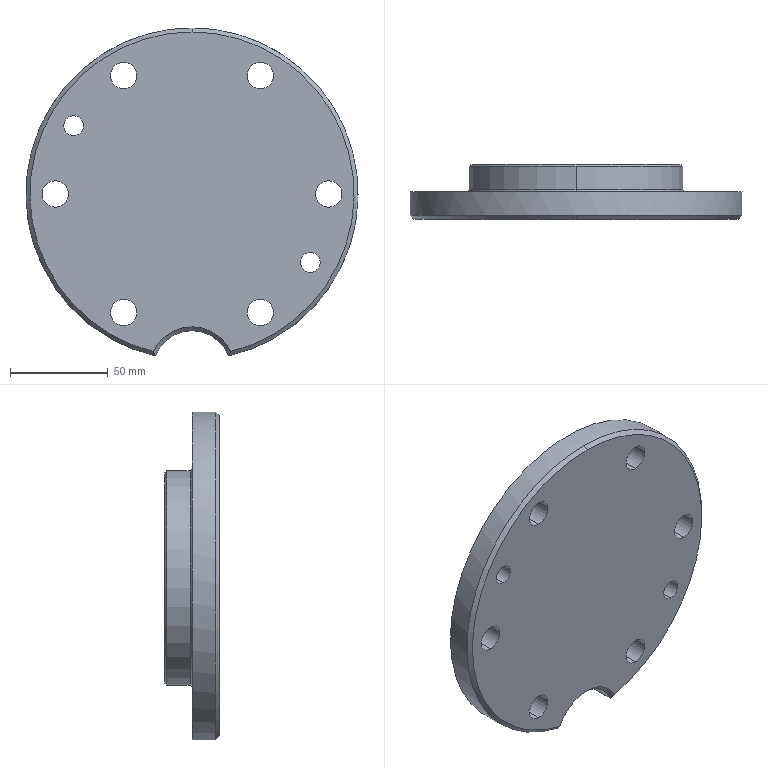Part | SolidWorks | features ICE 3, Chamfer 2, Fillet 2, Extrusion 1, HoleWzd 1 | 1 solid | 36 faces | box 170 x 28 x 167.917 mm | volume 262504 mm3 | cylinder 23 | cone 5 | torus 4 | plane 4 | commonest cylinder face diameters 13.5 x12 10.2 x4 40 x2 98 x2 110 x2 170 x1
STEP:
#1=CARTESIAN_POINT('',(0.,0.,83.));
#2=VERTEX_POINT('',#1);
#3=CARTESIAN_POINT('',(-19.883,0.,-80.583));
#4=VERTEX_POINT('',#3);
#5=CARTESIAN_POINT('',(0.,0.,0.));
#6=DIRECTION('',(0.,-1.,0.));
#7=DIRECTION('',(0.,0.,1.));
#8=AXIS2_PLACEMENT_3D('',#5,#6,#7);
#9=CIRCLE('',#8,83.);
#10=EDGE_CURVE('',#2,#4,#9,.T.);
#11=ORIENTED_EDGE('',*,*,#10,.F.);
#12=CARTESIAN_POINT('',(0.,2.,85.));
#13=VERTEX_POINT('',#12);
#14=CARTESIAN_POINT('',(0.,2.,85.));
#15=DIRECTION('',(0.,0.7071,0.7071));
#16=VECTOR('',#15,1000.);
#17=LINE('',#14,#16);
#18=EDGE_CURVE('',#2,#13,#17,.T.);
#19=ORIENTED_EDGE('',*,*,#18,.T.);
#20=CARTESIAN_POINT('',(-18.704,2.,-82.917));
#21=VERTEX_POINT('',#20);
#22=CARTESIAN_POINT('',(0.,2.,0.));
#23=DIRECTION('',(0.,1.,0.));
#24=DIRECTION('',(0.,0.,1.));
#25=AXIS2_PLACEMENT_3D('',#22,#23,#24);
#26=CIRCLE('',#25,85.);
#27=EDGE_CURVE('',#21,#13,#26,.T.);
#28=ORIENTED_EDGE('',*,*,#27,.F.);
#29=CARTESIAN_POINT('',(-19.883,0.,-80.583));
#30=CARTESIAN_POINT('',(-19.511,0.6719,-81.367));
#31=CARTESIAN_POINT('',(-19.119,1.339,-82.145));
#32=CARTESIAN_POINT('',(-18.704,2.,-82.917));
#33=B_SPLINE_CURVE_WITH_KNOTS('',3,(#29,#30,#31,#32),.UNSPECIFIED.,.F.,.F.,(4,4),(0.,0.003292),.UNSPECIFIED.);
#34=EDGE_CURVE('',#4,#21,#33,.T.);
#35=ORIENTED_EDGE('',*,*,#34,.F.);
#36=EDGE_LOOP('',(#11,#19,#28,#35));
#37=FACE_OUTER_BOUND('',#36,.T.);
#38=CARTESIAN_POINT('',(0.,2.,0.));
#39=DIRECTION('',(0.,1.,0.));
#40=DIRECTION('',(0.,0.,1.));
#41=AXIS2_PLACEMENT_3D('',#38,#39,#40);
#42=CONICAL_SURFACE('',#41,85.,0.7854);
#43=ADVANCED_FACE('',(#37),#42,.T.);
#44=CARTESIAN_POINT('',(-60.622,0.,29.9));
#45=VERTEX_POINT('',#44);
#46=CARTESIAN_POINT('',(-60.622,0.,40.1));
#47=VERTEX_POINT('',#46);
#48=CARTESIAN_POINT('',(-60.622,0.,35.));
#49=DIRECTION('',(0.,1.,0.));
#50=DIRECTION('',(0.,0.,1.));
#51=AXIS2_PLACEMENT_3D('',#48,#49,#50);
#52=CIRCLE('',#51,5.1);
#53=EDGE_CURVE('',#45,#47,#52,.T.);
#54=ORIENTED_EDGE('',*,*,#53,.F.);
#55=CARTESIAN_POINT('',(-60.622,14.,29.9));
#56=VERTEX_POINT('',#55);
#57=CARTESIAN_POINT('',(-60.622,14.,29.9));
#58=DIRECTION('',(0.,1.,0.));
#59=VECTOR('',#58,1000.);
#60=LINE('',#57,#59);
#61=EDGE_CURVE('',#45,#56,#60,.T.);
#62=ORIENTED_EDGE('',*,*,#61,.T.);
#63=CARTESIAN_POINT('',(-60.622,14.,40.1));
#64=VERTEX_POINT('',#63);
#65=CARTESIAN_POINT('',(-60.622,14.,35.));
#66=DIRECTION('',(0.,1.,0.));
#67=DIRECTION('',(0.,0.,1.));
#68=AXIS2_PLACEMENT_3D('',#65,#66,#67);
#69=CIRCLE('',#68,5.1);
#70=EDGE_CURVE('',#56,#64,#69,.T.);
#71=ORIENTED_EDGE('',*,*,#70,.T.);
#72=CARTESIAN_POINT('',(-60.622,14.,40.1));
#73=DIRECTION('',(0.,1.,0.));
#74=VECTOR('',#73,1000.);
#75=LINE('',#72,#74);
#76=EDGE_CURVE('',#47,#64,#75,.T.);
#77=ORIENTED_EDGE('',*,*,#76,.F.);
#78=EDGE_LOOP('',(#54,#62,#71,#77));
#79=FACE_OUTER_BOUND('',#78,.T.);
#80=CARTESIAN_POINT('',(-60.622,14.,35.));
#81=DIRECTION('',(0.,1.,0.));
#82=DIRECTION('',(0.,0.,1.));
#83=AXIS2_PLACEMENT_3D('',#80,#81,#82);
#84=CYLINDRICAL_SURFACE('',#83,5.1);
#85=ADVANCED_FACE('',(#79),#84,.F.);
#86=CARTESIAN_POINT('',(60.622,0.,-40.1));
#87=VERTEX_POINT('',#86);
#88=CARTESIAN_POINT('',(60.622,0.,-29.9));
#89=VERTEX_POINT('',#88);
#90=CARTESIAN_POINT('',(60.622,0.,-35.));
#91=DIRECTION('',(0.,1.,0.));
#92=DIRECTION('',(0.,0.,1.));
#93=AXIS2_PLACEMENT_3D('',#90,#91,#92);
#94=CIRCLE('',#93,5.1);
#95=EDGE_CURVE('',#87,#89,#94,.T.);
#96=ORIENTED_EDGE('',*,*,#95,.F.);
#97=CARTESIAN_POINT('',(60.622,14.,-40.1));
#98=VERTEX_POINT('',#97);
#99=CARTESIAN_POINT('',(60.622,14.,-40.1));
#100=DIRECTION('',(0.,1.,0.));
#101=VECTOR('',#100,1000.);
#102=LINE('',#99,#101);
#103=EDGE_CURVE('',#87,#98,#102,.T.);
#104=ORIENTED_EDGE('',*,*,#103,.T.);
#105=CARTESIAN_POINT('',(60.622,14.,-29.9));
#106=VERTEX_POINT('',#105);
#107=CARTESIAN_POINT('',(60.622,14.,-35.));
#108=DIRECTION('',(0.,1.,0.));
#109=DIRECTION('',(0.,0.,1.));
#110=AXIS2_PLACEMENT_3D('',#107,#108,#109);
#111=CIRCLE('',#110,5.1);
#112=EDGE_CURVE('',#98,#106,#111,.T.);
#113=ORIENTED_EDGE('',*,*,#112,.T.);
#114=CARTESIAN_POINT('',(60.622,14.,-29.9));
#115=DIRECTION('',(0.,1.,0.));
#116=VECTOR('',#115,1000.);
#117=LINE('',#114,#116);
#118=EDGE_CURVE('',#89,#106,#117,.T.);
#119=ORIENTED_EDGE('',*,*,#118,.F.);
#120=EDGE_LOOP('',(#96,#104,#113,#119));
#121=FACE_OUTER_BOUND('',#120,.T.);
#122=CARTESIAN_POINT('',(60.622,14.,-35.));
#123=DIRECTION('',(0.,1.,0.));
#124=DIRECTION('',(0.,0.,1.));
#125=AXIS2_PLACEMENT_3D('',#122,#123,#124);
#126=CYLINDRICAL_SURFACE('',#125,5.1);
#127=ADVANCED_FACE('',(#121),#126,.F.);
#128=CARTESIAN_POINT('',(18.704,2.,-82.917));
#129=VERTEX_POINT('',#128);
#130=CARTESIAN_POINT('',(0.,2.,-70.));
#131=VERTEX_POINT('',#130);
#132=CARTESIAN_POINT('',(0.,2.,-90.));
#133=DIRECTION('',(0.,-1.,0.));
#134=DIRECTION('',(0.,0.,1.));
#135=AXIS2_PLACEMENT_3D('',#132,#133,#134);
#136=CIRCLE('',#135,20.);
#137=EDGE_CURVE('',#129,#131,#136,.T.);
#138=ORIENTED_EDGE('',*,*,#137,.T.);
#139=CARTESIAN_POINT('',(0.,14.,-70.));
#140=VERTEX_POINT('',#139);
#141=CARTESIAN_POINT('',(0.,0.,-70.));
#142=DIRECTION('',(0.,1.,0.));
#143=VECTOR('',#142,1000.);
#144=LINE('',#141,#143);
#145=EDGE_CURVE('',#131,#140,#144,.T.);
#146=ORIENTED_EDGE('',*,*,#145,.T.);
#147=CARTESIAN_POINT('',(18.704,14.,-82.917));
#148=VERTEX_POINT('',#147);
#149=CARTESIAN_POINT('',(0.,14.,-90.));
#150=DIRECTION('',(0.,1.,0.));
#151=DIRECTION('',(0.,0.,1.));
#152=AXIS2_PLACEMENT_3D('',#149,#150,#151);
#153=CIRCLE('',#152,20.);
#154=EDGE_CURVE('',#140,#148,#153,.T.);
#155=ORIENTED_EDGE('',*,*,#154,.T.);
#156=CARTESIAN_POINT('',(18.704,7.,-82.917));
#157=DIRECTION('',(0.,1.,0.));
#158=VECTOR('',#157,1000.);
#159=LINE('',#156,#158);
#160=EDGE_CURVE('',#129,#148,#159,.T.);
#161=ORIENTED_EDGE('',*,*,#160,.F.);
#162=EDGE_LOOP('',(#138,#146,#155,#161));
#163=FACE_OUTER_BOUND('',#162,.T.);
#164=CARTESIAN_POINT('',(0.,0.,-90.));
#165=DIRECTION('',(0.,1.,0.));
#166=DIRECTION('',(0.,0.,1.));
#167=AXIS2_PLACEMENT_3D('',#164,#165,#166);
#168=CYLINDRICAL_SURFACE('',#167,20.);
#169=ADVANCED_FACE('',(#163),#168,.F.);
#170=CARTESIAN_POINT('',(-70.,0.,-6.75));
#171=VERTEX_POINT('',#170);
#172=CARTESIAN_POINT('',(-70.,0.,6.75));
#173=VERTEX_POINT('',#172);
#174=CARTESIAN_POINT('',(-70.,0.,0.));
#175=DIRECTION('',(0.,1.,0.));
#176=DIRECTION('',(0.,0.,1.));
#177=AXIS2_PLACEMENT_3D('',#174,#175,#176);
#178=CIRCLE('',#177,6.75);
#179=EDGE_CURVE('',#171,#173,#178,.T.);
#180=ORIENTED_EDGE('',*,*,#179,.F.);
#181=CARTESIAN_POINT('',(-70.,14.,-6.75));
#182=VERTEX_POINT('',#181);
#183=CARTESIAN_POINT('',(-70.,0.,-6.75));
#184=DIRECTION('',(0.,1.,0.));
#185=VECTOR('',#184,1000.);
#186=LINE('',#183,#185);
#187=EDGE_CURVE('',#171,#182,#186,.T.);
#188=ORIENTED_EDGE('',*,*,#187,.T.);
#189=CARTESIAN_POINT('',(-70.,14.,6.75));
#190=VERTEX_POINT('',#189);
#191=CARTESIAN_POINT('',(-70.,14.,0.));
#192=DIRECTION('',(0.,1.,0.));
#193=DIRECTION('',(0.,0.,1.));
#194=AXIS2_PLACEMENT_3D('',#191,#192,#193);
#195=CIRCLE('',#194,6.75);
#196=EDGE_CURVE('',#182,#190,#195,.T.);
#197=ORIENTED_EDGE('',*,*,#196,.T.);
#198=CARTESIAN_POINT('',(-70.,0.,6.75));
#199=DIRECTION('',(0.,1.,0.));
#200=VECTOR('',#199,1000.);
#201=LINE('',#198,#200);
#202=EDGE_CURVE('',#173,#190,#201,.T.);
#203=ORIENTED_EDGE('',*,*,#202,.F.);
#204=EDGE_LOOP('',(#180,#188,#197,#203));
#205=FACE_OUTER_BOUND('',#204,.T.);
#206=CARTESIAN_POINT('',(-70.,0.,0.));
#207=DIRECTION('',(0.,1.,0.));
#208=DIRECTION('',(0.,0.,1.));
#209=AXIS2_PLACEMENT_3D('',#206,#207,#208);
#210=CYLINDRICAL_SURFACE('',#209,6.75);
#211=ADVANCED_FACE('',(#205),#210,.F.);
#212=CARTESIAN_POINT('',(-35.,0.,53.872));
#213=VERTEX_POINT('',#212);
#214=CARTESIAN_POINT('',(-35.,0.,67.372));
#215=VERTEX_POINT('',#214);
#216=CARTESIAN_POINT('',(-35.,0.,60.622));
#217=DIRECTION('',(0.,1.,0.));
#218=DIRECTION('',(0.,0.,1.));
#219=AXIS2_PLACEMENT_3D('',#216,#217,#218);
#220=CIRCLE('',#219,6.75);
#221=EDGE_CURVE('',#213,#215,#220,.T.);
#222=ORIENTED_EDGE('',*,*,#221,.F.);
#223=CARTESIAN_POINT('',(-35.,14.,53.872));
#224=VERTEX_POINT('',#223);
#225=CARTESIAN_POINT('',(-35.,0.,53.872));
#226=DIRECTION('',(0.,1.,0.));
#227=VECTOR('',#226,1000.);
#228=LINE('',#225,#227);
#229=EDGE_CURVE('',#213,#224,#228,.T.);
#230=ORIENTED_EDGE('',*,*,#229,.T.);
#231=CARTESIAN_POINT('',(-35.,14.,67.372));
#232=VERTEX_POINT('',#231);
#233=CARTESIAN_POINT('',(-35.,14.,60.622));
#234=DIRECTION('',(0.,1.,0.));
#235=DIRECTION('',(0.,0.,1.));
#236=AXIS2_PLACEMENT_3D('',#233,#234,#235);
#237=CIRCLE('',#236,6.75);
#238=EDGE_CURVE('',#224,#232,#237,.T.);
#239=ORIENTED_EDGE('',*,*,#238,.T.);
#240=CARTESIAN_POINT('',(-35.,0.,67.372));
#241=DIRECTION('',(0.,1.,0.));
#242=VECTOR('',#241,1000.);
#243=LINE('',#240,#242);
#244=EDGE_CURVE('',#215,#232,#243,.T.);
#245=ORIENTED_EDGE('',*,*,#244,.F.);
#246=EDGE_LOOP('',(#222,#230,#239,#245));
#247=FACE_OUTER_BOUND('',#246,.T.);
#248=CARTESIAN_POINT('',(-35.,0.,60.622));
#249=DIRECTION('',(0.,1.,0.));
#250=DIRECTION('',(0.,0.,1.));
#251=AXIS2_PLACEMENT_3D('',#248,#249,#250);
#252=CYLINDRICAL_SURFACE('',#251,6.75);
#253=ADVANCED_FACE('',(#247),#252,.F.);
#254=CARTESIAN_POINT('',(35.,0.,53.872));
#255=VERTEX_POINT('',#254);
#256=CARTESIAN_POINT('',(35.,0.,67.372));
#257=VERTEX_POINT('',#256);
#258=CARTESIAN_POINT('',(35.,0.,60.622));
#259=DIRECTION('',(0.,1.,0.));
#260=DIRECTION('',(0.,0.,1.));
#261=AXIS2_PLACEMENT_3D('',#258,#259,#260);
#262=CIRCLE('',#261,6.75);
#263=EDGE_CURVE('',#255,#257,#262,.T.);
#264=ORIENTED_EDGE('',*,*,#263,.F.);
#265=CARTESIAN_POINT('',(35.,14.,53.872));
#266=VERTEX_POINT('',#265);
#267=CARTESIAN_POINT('',(35.,0.,53.872));
#268=DIRECTION('',(0.,1.,0.));
#269=VECTOR('',#268,1000.);
#270=LINE('',#267,#269);
#271=EDGE_CURVE('',#255,#266,#270,.T.);
#272=ORIENTED_EDGE('',*,*,#271,.T.);
#273=CARTESIAN_POINT('',(35.,14.,67.372));
#274=VERTEX_POINT('',#273);
#275=CARTESIAN_POINT('',(35.,14.,60.622));
#276=DIRECTION('',(0.,1.,0.));
#277=DIRECTION('',(0.,0.,1.));
#278=AXIS2_PLACEMENT_3D('',#275,#276,#277);
#279=CIRCLE('',#278,6.75);
#280=EDGE_CURVE('',#266,#274,#279,.T.);
#281=ORIENTED_EDGE('',*,*,#280,.T.);
#282=CARTESIAN_POINT('',(35.,0.,67.372));
#283=DIRECTION('',(0.,1.,0.));
#284=VECTOR('',#283,1000.);
#285=LINE('',#282,#284);
#286=EDGE_CURVE('',#257,#274,#285,.T.);
#287=ORIENTED_EDGE('',*,*,#286,.F.);
#288=EDGE_LOOP('',(#264,#272,#281,#287));
#289=FACE_OUTER_BOUND('',#288,.T.);
#290=CARTESIAN_POINT('',(35.,0.,60.622));
#291=DIRECTION('',(0.,1.,0.));
#292=DIRECTION('',(0.,0.,1.));
#293=AXIS2_PLACEMENT_3D('',#290,#291,#292);
#294=CYLINDRICAL_SURFACE('',#293,6.75);
#295=ADVANCED_FACE('',(#289),#294,.F.);
#296=CARTESIAN_POINT('',(70.,0.,-6.75));
#297=VERTEX_POINT('',#296);
#298=CARTESIAN_POINT('',(70.,0.,6.75));
#299=VERTEX_POINT('',#298);
#300=CARTESIAN_POINT('',(70.,0.,0.));
#301=DIRECTION('',(0.,1.,0.));
#302=DIRECTION('',(0.,0.,1.));
#303=AXIS2_PLACEMENT_3D('',#300,#301,#302);
#304=CIRCLE('',#303,6.75);
#305=EDGE_CURVE('',#297,#299,#304,.T.);
#306=ORIENTED_EDGE('',*,*,#305,.F.);
#307=CARTESIAN_POINT('',(70.,14.,-6.75));
#308=VERTEX_POINT('',#307);
#309=CARTESIAN_POINT('',(70.,0.,-6.75));
#310=DIRECTION('',(0.,1.,0.));
#311=VECTOR('',#310,1000.);
#312=LINE('',#309,#311);
#313=EDGE_CURVE('',#297,#308,#312,.T.);
#314=ORIENTED_EDGE('',*,*,#313,.T.);
#315=CARTESIAN_POINT('',(70.,14.,6.75));
#316=VERTEX_POINT('',#315);
#317=CARTESIAN_POINT('',(70.,14.,0.));
#318=DIRECTION('',(0.,1.,0.));
#319=DIRECTION('',(0.,0.,1.));
#320=AXIS2_PLACEMENT_3D('',#317,#318,#319);
#321=CIRCLE('',#320,6.75);
#322=EDGE_CURVE('',#308,#316,#321,.T.);
#323=ORIENTED_EDGE('',*,*,#322,.T.);
#324=CARTESIAN_POINT('',(70.,0.,6.75));
#325=DIRECTION('',(0.,1.,0.));
#326=VECTOR('',#325,1000.);
#327=LINE('',#324,#326);
#328=EDGE_CURVE('',#299,#316,#327,.T.);
#329=ORIENTED_EDGE('',*,*,#328,.F.);
#330=EDGE_LOOP('',(#306,#314,#323,#329));
#331=FACE_OUTER_BOUND('',#330,.T.);
#332=CARTESIAN_POINT('',(70.,0.,0.));
#333=DIRECTION('',(0.,1.,0.));
#334=DIRECTION('',(0.,0.,1.));
#335=AXIS2_PLACEMENT_3D('',#332,#333,#334);
#336=CYLINDRICAL_SURFACE('',#335,6.75);
#337=ADVANCED_FACE('',(#331),#336,.F.);
#338=CARTESIAN_POINT('',(35.,0.,-67.372));
#339=VERTEX_POINT('',#338);
#340=CARTESIAN_POINT('',(35.,0.,-53.872));
#341=VERTEX_POINT('',#340);
#342=CARTESIAN_POINT('',(35.,0.,-60.622));
#343=DIRECTION('',(0.,1.,0.));
#344=DIRECTION('',(0.,0.,1.));
#345=AXIS2_PLACEMENT_3D('',#342,#343,#344);
#346=CIRCLE('',#345,6.75);
#347=EDGE_CURVE('',#339,#341,#346,.T.);
#348=ORIENTED_EDGE('',*,*,#347,.F.);
#349=CARTESIAN_POINT('',(35.,14.,-67.372));
#350=VERTEX_POINT('',#349);
#351=CARTESIAN_POINT('',(35.,0.,-67.372));
#352=DIRECTION('',(0.,1.,0.));
#353=VECTOR('',#352,1000.);
#354=LINE('',#351,#353);
#355=EDGE_CURVE('',#339,#350,#354,.T.);
#356=ORIENTED_EDGE('',*,*,#355,.T.);
#357=CARTESIAN_POINT('',(35.,14.,-53.872));
#358=VERTEX_POINT('',#357);
#359=CARTESIAN_POINT('',(35.,14.,-60.622));
#360=DIRECTION('',(0.,1.,0.));
#361=DIRECTION('',(0.,0.,1.));
#362=AXIS2_PLACEMENT_3D('',#359,#360,#361);
#363=CIRCLE('',#362,6.75);
#364=EDGE_CURVE('',#350,#358,#363,.T.);
#365=ORIENTED_EDGE('',*,*,#364,.T.);
#366=CARTESIAN_POINT('',(35.,0.,-53.872));
#367=DIRECTION('',(0.,1.,0.));
#368=VECTOR('',#367,1000.);
#369=LINE('',#366,#368);
#370=EDGE_CURVE('',#341,#358,#369,.T.);
#371=ORIENTED_EDGE('',*,*,#370,.F.);
#372=EDGE_LOOP('',(#348,#356,#365,#371));
#373=FACE_OUTER_BOUND('',#372,.T.);
#374=CARTESIAN_POINT('',(35.,0.,-60.622));
#375=DIRECTION('',(0.,1.,0.));
#376=DIRECTION('',(0.,0.,1.));
#377=AXIS2_PLACEMENT_3D('',#374,#375,#376);
#378=CYLINDRICAL_SURFACE('',#377,6.75);
#379=ADVANCED_FACE('',(#373),#378,.F.);
#380=CARTESIAN_POINT('',(-35.,0.,-67.372));
#381=VERTEX_POINT('',#380);
#382=CARTESIAN_POINT('',(-35.,0.,-53.872));
#383=VERTEX_POINT('',#382);
#384=CARTESIAN_POINT('',(-35.,0.,-60.622));
#385=DIRECTION('',(0.,1.,0.));
#386=DIRECTION('',(0.,0.,1.));
#387=AXIS2_PLACEMENT_3D('',#384,#385,#386);
#388=CIRCLE('',#387,6.75);
#389=EDGE_CURVE('',#381,#383,#388,.T.);
#390=ORIENTED_EDGE('',*,*,#389,.F.);
#391=CARTESIAN_POINT('',(-35.,14.,-67.372));
#392=VERTEX_POINT('',#391);
#393=CARTESIAN_POINT('',(-35.,0.,-67.372));
#394=DIRECTION('',(0.,1.,0.));
#395=VECTOR('',#394,1000.);
#396=LINE('',#393,#395);
#397=EDGE_CURVE('',#381,#392,#396,.T.);
#398=ORIENTED_EDGE('',*,*,#397,.T.);
#399=CARTESIAN_POINT('',(-35.,14.,-53.872));
#400=VERTEX_POINT('',#399);
#401=CARTESIAN_POINT('',(-35.,14.,-60.622));
#402=DIRECTION('',(0.,1.,0.));
#403=DIRECTION('',(0.,0.,1.));
#404=AXIS2_PLACEMENT_3D('',#401,#402,#403);
#405=CIRCLE('',#404,6.75);
#406=EDGE_CURVE('',#392,#400,#405,.T.);
#407=ORIENTED_EDGE('',*,*,#406,.T.);
#408=CARTESIAN_POINT('',(-35.,0.,-53.872));
#409=DIRECTION('',(0.,1.,0.));
#410=VECTOR('',#409,1000.);
#411=LINE('',#408,#410);
#412=EDGE_CURVE('',#383,#400,#411,.T.);
#413=ORIENTED_EDGE('',*,*,#412,.F.);
#414=EDGE_LOOP('',(#390,#398,#407,#413));
#415=FACE_OUTER_BOUND('',#414,.T.);
#416=CARTESIAN_POINT('',(-35.,0.,-60.622));
#417=DIRECTION('',(0.,1.,0.));
#418=DIRECTION('',(0.,0.,1.));
#419=AXIS2_PLACEMENT_3D('',#416,#417,#418);
#420=CYLINDRICAL_SURFACE('',#419,6.75);
#421=ADVANCED_FACE('',(#415),#420,.F.);
#422=CARTESIAN_POINT('',(0.,28.,54.));
#423=VERTEX_POINT('',#422);
#424=CARTESIAN_POINT('',(0.,28.,-54.));
#425=VERTEX_POINT('',#424);
#426=CARTESIAN_POINT('',(0.,28.,0.));
#427=DIRECTION('',(0.,1.,0.));
#428=DIRECTION('',(0.,0.,1.));
#429=AXIS2_PLACEMENT_3D('',#426,#427,#428);
#430=CIRCLE('',#429,54.);
#431=EDGE_CURVE('',#423,#425,#430,.T.);
#432=ORIENTED_EDGE('',*,*,#431,.F.);
#433=CARTESIAN_POINT('',(0.,27.,55.));
#434=VERTEX_POINT('',#433);
#435=CARTESIAN_POINT('',(0.,28.,54.));
#436=DIRECTION('',(0.,-0.7071,0.7071));
#437=VECTOR('',#436,1000.);
#438=LINE('',#435,#437);
#439=EDGE_CURVE('',#423,#434,#438,.T.);
#440=ORIENTED_EDGE('',*,*,#439,.T.);
#441=CARTESIAN_POINT('',(0.,27.,-55.));
#442=VERTEX_POINT('',#441);
#443=CARTESIAN_POINT('',(0.,27.,0.));
#444=DIRECTION('',(0.,-1.,0.));
#445=DIRECTION('',(0.,0.,1.));
#446=AXIS2_PLACEMENT_3D('',#443,#444,#445);
#447=CIRCLE('',#446,55.);
#448=EDGE_CURVE('',#442,#434,#447,.T.);
#449=ORIENTED_EDGE('',*,*,#448,.F.);
#450=CARTESIAN_POINT('',(0.,28.,-54.));
#451=DIRECTION('',(0.,-0.7071,-0.7071));
#452=VECTOR('',#451,1000.);
#453=LINE('',#450,#452);
#454=EDGE_CURVE('',#425,#442,#453,.T.);
#455=ORIENTED_EDGE('',*,*,#454,.F.);
#456=EDGE_LOOP('',(#432,#440,#449,#455));
#457=FACE_OUTER_BOUND('',#456,.T.);
#458=CARTESIAN_POINT('',(0.,28.,0.));
#459=DIRECTION('',(0.,-1.,0.));
#460=DIRECTION('',(0.,0.,-1.));
#461=AXIS2_PLACEMENT_3D('',#458,#459,#460);
#462=CONICAL_SURFACE('',#461,54.,0.7854);
#463=ADVANCED_FACE('',(#457),#462,.T.);
#464=CARTESIAN_POINT('',(0.,15.,-55.));
#465=VERTEX_POINT('',#464);
#466=CARTESIAN_POINT('',(0.,15.,55.));
#467=VERTEX_POINT('',#466);
#468=CARTESIAN_POINT('',(0.,15.,0.));
#469=DIRECTION('',(0.,1.,0.));
#470=DIRECTION('',(0.,0.,1.));
#471=AXIS2_PLACEMENT_3D('',#468,#469,#470);
#472=CIRCLE('',#471,55.);
#473=EDGE_CURVE('',#465,#467,#472,.T.);
#474=ORIENTED_EDGE('',*,*,#473,.F.);
#475=CARTESIAN_POINT('',(0.,14.,-56.));
#476=VERTEX_POINT('',#475);
#477=CARTESIAN_POINT('',(0.,15.,-56.));
#478=DIRECTION('',(1.,0.,0.));
#479=DIRECTION('',(0.,0.,-1.));
#480=AXIS2_PLACEMENT_3D('',#477,#478,#479);
#481=CIRCLE('',#480,1.);
#482=EDGE_CURVE('',#465,#476,#481,.T.);
#483=ORIENTED_EDGE('',*,*,#482,.T.);
#484=CARTESIAN_POINT('',(0.,14.,56.));
#485=VERTEX_POINT('',#484);
#486=CARTESIAN_POINT('',(0.,14.,0.));
#487=DIRECTION('',(0.,-1.,0.));
#488=DIRECTION('',(0.,0.,1.));
#489=AXIS2_PLACEMENT_3D('',#486,#487,#488);
#490=CIRCLE('',#489,56.);
#491=EDGE_CURVE('',#485,#476,#490,.T.);
#492=ORIENTED_EDGE('',*,*,#491,.F.);
#493=CARTESIAN_POINT('',(0.,15.,56.));
#494=DIRECTION('',(-1.,0.,0.));
#495=DIRECTION('',(0.,0.,1.));
#496=AXIS2_PLACEMENT_3D('',#493,#494,#495);
#497=CIRCLE('',#496,1.);
#498=EDGE_CURVE('',#467,#485,#497,.T.);
#499=ORIENTED_EDGE('',*,*,#498,.F.);
#500=EDGE_LOOP('',(#474,#483,#492,#499));
#501=FACE_OUTER_BOUND('',#500,.T.);
#502=CARTESIAN_POINT('',(0.,15.,0.));
#503=DIRECTION('',(0.,1.,0.));
#504=DIRECTION('',(0.,0.,1.));
#505=AXIS2_PLACEMENT_3D('',#502,#503,#504);
#506=TOROIDAL_SURFACE('',#505,56.,1.);
#507=ADVANCED_FACE('',(#501),#506,.F.);
#508=CARTESIAN_POINT('',(0.,5.,-39.));
#509=VERTEX_POINT('',#508);
#510=CARTESIAN_POINT('',(0.,5.,39.));
#511=VERTEX_POINT('',#510);
#512=CARTESIAN_POINT('',(0.,5.,0.));
#513=DIRECTION('',(0.,1.,0.));
#514=DIRECTION('',(0.,0.,1.));
#515=AXIS2_PLACEMENT_3D('',#512,#513,#514);
#516=CIRCLE('',#515,39.);
#517=EDGE_CURVE('',#509,#511,#516,.T.);
#518=ORIENTED_EDGE('',*,*,#517,.F.);
#519=CARTESIAN_POINT('',(0.,15.,-49.));
#520=VERTEX_POINT('',#519);
#521=CARTESIAN_POINT('',(0.,15.,-39.));
#522=DIRECTION('',(1.,0.,0.));
#523=DIRECTION('',(0.,0.,-1.));
#524=AXIS2_PLACEMENT_3D('',#521,#522,#523);
#525=CIRCLE('',#524,10.);
#526=EDGE_CURVE('',#509,#520,#525,.T.);
#527=ORIENTED_EDGE('',*,*,#526,.T.);
#528=CARTESIAN_POINT('',(0.,15.,49.));
#529=VERTEX_POINT('',#528);
#530=CARTESIAN_POINT('',(0.,15.,0.));
#531=DIRECTION('',(0.,-1.,0.));
#532=DIRECTION('',(0.,0.,1.));
#533=AXIS2_PLACEMENT_3D('',#530,#531,#532);
#534=CIRCLE('',#533,49.);
#535=EDGE_CURVE('',#529,#520,#534,.T.);
#536=ORIENTED_EDGE('',*,*,#535,.F.);
#537=CARTESIAN_POINT('',(0.,15.,39.));
#538=DIRECTION('',(-1.,0.,0.));
#539=DIRECTION('',(0.,0.,1.));
#540=AXIS2_PLACEMENT_3D('',#537,#538,#539);
#541=CIRCLE('',#540,10.);
#542=EDGE_CURVE('',#511,#529,#541,.T.);
#543=ORIENTED_EDGE('',*,*,#542,.F.);
#544=EDGE_LOOP('',(#518,#527,#536,#543));
#545=FACE_OUTER_BOUND('',#544,.T.);
#546=CARTESIAN_POINT('',(0.,15.,0.));
#547=DIRECTION('',(0.,1.,0.));
#548=DIRECTION('',(0.,0.,1.));
#549=AXIS2_PLACEMENT_3D('',#546,#547,#548);
#550=TOROIDAL_SURFACE('',#549,39.,10.);
#551=ADVANCED_FACE('',(#545),#550,.F.);
#552=ORIENTED_EDGE('',*,*,#535,.T.);
#553=CARTESIAN_POINT('',(0.,28.,-49.));
#554=VERTEX_POINT('',#553);
#555=CARTESIAN_POINT('',(0.,5.,-49.));
#556=DIRECTION('',(0.,1.,0.));
#557=VECTOR('',#556,1000.);
#558=LINE('',#555,#557);
#559=EDGE_CURVE('',#520,#554,#558,.T.);
#560=ORIENTED_EDGE('',*,*,#559,.T.);
#561=CARTESIAN_POINT('',(0.,28.,49.));
#562=VERTEX_POINT('',#561);
#563=CARTESIAN_POINT('',(0.,28.,0.));
#564=DIRECTION('',(0.,1.,0.));
#565=DIRECTION('',(0.,0.,1.));
#566=AXIS2_PLACEMENT_3D('',#563,#564,#565);
#567=CIRCLE('',#566,49.);
#568=EDGE_CURVE('',#554,#562,#567,.T.);
#569=ORIENTED_EDGE('',*,*,#568,.T.);
#570=CARTESIAN_POINT('',(0.,5.,49.));
#571=DIRECTION('',(0.,1.,0.));
#572=VECTOR('',#571,1000.);
#573=LINE('',#570,#572);
#574=EDGE_CURVE('',#529,#562,#573,.T.);
#575=ORIENTED_EDGE('',*,*,#574,.F.);
#576=EDGE_LOOP('',(#552,#560,#569,#575));
#577=FACE_OUTER_BOUND('',#576,.T.);
#578=CARTESIAN_POINT('',(0.,5.,0.));
#579=DIRECTION('',(0.,1.,0.));
#580=DIRECTION('',(0.,0.,1.));
#581=AXIS2_PLACEMENT_3D('',#578,#579,#580);
#582=CYLINDRICAL_SURFACE('',#581,49.);
#583=ADVANCED_FACE('',(#577),#582,.F.);
#584=ORIENTED_EDGE('',*,*,#448,.T.);
#585=CARTESIAN_POINT('',(0.,28.,55.));
#586=DIRECTION('',(0.,-1.,0.));
#587=VECTOR('',#586,1000.);
#588=LINE('',#585,#587);
#589=EDGE_CURVE('',#434,#467,#588,.T.);
#590=ORIENTED_EDGE('',*,*,#589,.T.);
#591=CARTESIAN_POINT('',(0.,15.,0.));
#592=DIRECTION('',(0.,1.,0.));
#593=DIRECTION('',(0.,0.,1.));
#594=AXIS2_PLACEMENT_3D('',#591,#592,#593);
#595=CIRCLE('',#594,55.);
#596=EDGE_CURVE('',#467,#465,#595,.T.);
#597=ORIENTED_EDGE('',*,*,#596,.T.);
#598=CARTESIAN_POINT('',(0.,28.,-55.));
#599=DIRECTION('',(0.,-1.,0.));
#600=VECTOR('',#599,1000.);
#601=LINE('',#598,#600);
#602=EDGE_CURVE('',#442,#465,#601,.T.);
#603=ORIENTED_EDGE('',*,*,#602,.F.);
#604=EDGE_LOOP('',(#584,#590,#597,#603));
#605=FACE_OUTER_BOUND('',#604,.T.);
#606=CARTESIAN_POINT('',(0.,28.,0.));
#607=DIRECTION('',(0.,-1.,0.));
#608=DIRECTION('',(0.,0.,-1.));
#609=AXIS2_PLACEMENT_3D('',#606,#607,#608);
#610=CYLINDRICAL_SURFACE('',#609,55.);
#611=ADVANCED_FACE('',(#605),#610,.T.);
#612=CARTESIAN_POINT('',(-18.704,14.,-82.917));
#613=VERTEX_POINT('',#612);
#614=CARTESIAN_POINT('',(-18.704,7.,-82.917));
#615=DIRECTION('',(0.,-1.,0.));
#616=VECTOR('',#615,1000.);
#617=LINE('',#614,#616);
#618=EDGE_CURVE('',#613,#21,#617,.T.);
#619=ORIENTED_EDGE('',*,*,#618,.T.);
#620=ORIENTED_EDGE('',*,*,#27,.T.);
#621=CARTESIAN_POINT('',(0.,2.,0.));
#622=DIRECTION('',(0.,1.,0.));
#623=DIRECTION('',(0.,0.,1.));
#624=AXIS2_PLACEMENT_3D('',#621,#622,#623);
#625=CIRCLE('',#624,85.);
#626=EDGE_CURVE('',#13,#129,#625,.T.);
#627=ORIENTED_EDGE('',*,*,#626,.T.);
#628=ORIENTED_EDGE('',*,*,#160,.T.);
#629=CARTESIAN_POINT('',(0.,14.,0.));
#630=DIRECTION('',(0.,1.,0.));
#631=DIRECTION('',(0.,0.,1.));
#632=AXIS2_PLACEMENT_3D('',#629,#630,#631);
#633=CIRCLE('',#632,85.);
#634=EDGE_CURVE('',#613,#148,#633,.T.);
#635=ORIENTED_EDGE('',*,*,#634,.F.);
#636=EDGE_LOOP('',(#619,#620,#627,#628,#635));
#637=FACE_OUTER_BOUND('',#636,.T.);
#638=CARTESIAN_POINT('',(0.,14.,0.));
#639=DIRECTION('',(0.,-1.,0.));
#640=DIRECTION('',(0.,0.,-1.));
#641=AXIS2_PLACEMENT_3D('',#638,#639,#640);
#642=CYLINDRICAL_SURFACE('',#641,85.);
#643=ADVANCED_FACE('',(#637),#642,.T.);
#644=CARTESIAN_POINT('',(-60.622,14.,35.));
#645=DIRECTION('',(0.,1.,0.));
#646=DIRECTION('',(0.,0.,1.));
#647=AXIS2_PLACEMENT_3D('',#644,#645,#646);
#648=CIRCLE('',#647,5.1);
#649=EDGE_CURVE('',#64,#56,#648,.T.);
#650=ORIENTED_EDGE('',*,*,#649,.F.);
#651=ORIENTED_EDGE('',*,*,#70,.F.);
#652=EDGE_LOOP('',(#650,#651));
#653=FACE_BOUND('',#652,.T.);
#654=CARTESIAN_POINT('',(60.622,14.,-35.));
#655=DIRECTION('',(0.,1.,0.));
#656=DIRECTION('',(0.,0.,1.));
#657=AXIS2_PLACEMENT_3D('',#654,#655,#656);
#658=CIRCLE('',#657,5.1);
#659=EDGE_CURVE('',#106,#98,#658,.T.);
#660=ORIENTED_EDGE('',*,*,#659,.F.);
#661=ORIENTED_EDGE('',*,*,#112,.F.);
#662=EDGE_LOOP('',(#660,#661));
#663=FACE_BOUND('',#662,.T.);
#664=CARTESIAN_POINT('',(0.,14.,-90.));
#665=DIRECTION('',(0.,1.,0.));
#666=DIRECTION('',(0.,0.,1.));
#667=AXIS2_PLACEMENT_3D('',#664,#665,#666);
#668=CIRCLE('',#667,20.);
#669=EDGE_CURVE('',#613,#140,#668,.T.);
#670=ORIENTED_EDGE('',*,*,#669,.F.);
#671=ORIENTED_EDGE('',*,*,#634,.T.);
#672=ORIENTED_EDGE('',*,*,#154,.F.);
#673=EDGE_LOOP('',(#670,#671,#672));
#674=FACE_OUTER_BOUND('',#673,.T.);
#675=CARTESIAN_POINT('',(-70.,14.,0.));
#676=DIRECTION('',(0.,1.,0.));
#677=DIRECTION('',(0.,0.,1.));
#678=AXIS2_PLACEMENT_3D('',#675,#676,#677);
#679=CIRCLE('',#678,6.75);
#680=EDGE_CURVE('',#190,#182,#679,.T.);
#681=ORIENTED_EDGE('',*,*,#680,.F.);
#682=ORIENTED_EDGE('',*,*,#196,.F.);
#683=EDGE_LOOP('',(#681,#682));
#684=FACE_BOUND('',#683,.T.);
#685=CARTESIAN_POINT('',(-35.,14.,60.622));
#686=DIRECTION('',(0.,1.,0.));
#687=DIRECTION('',(0.,0.,1.));
#688=AXIS2_PLACEMENT_3D('',#685,#686,#687);
#689=CIRCLE('',#688,6.75);
#690=EDGE_CURVE('',#232,#224,#689,.T.);
#691=ORIENTED_EDGE('',*,*,#690,.F.);
#692=ORIENTED_EDGE('',*,*,#238,.F.);
#693=EDGE_LOOP('',(#691,#692));
#694=FACE_BOUND('',#693,.T.);
#695=CARTESIAN_POINT('',(35.,14.,60.622));
#696=DIRECTION('',(0.,1.,0.));
#697=DIRECTION('',(0.,0.,1.));
#698=AXIS2_PLACEMENT_3D('',#695,#696,#697);
#699=CIRCLE('',#698,6.75);
#700=EDGE_CURVE('',#274,#266,#699,.T.);
#701=ORIENTED_EDGE('',*,*,#700,.F.);
#702=ORIENTED_EDGE('',*,*,#280,.F.);
#703=EDGE_LOOP('',(#701,#702));
#704=FACE_BOUND('',#703,.T.);
#705=CARTESIAN_POINT('',(70.,14.,0.));
#706=DIRECTION('',(0.,1.,0.));
#707=DIRECTION('',(0.,0.,1.));
#708=AXIS2_PLACEMENT_3D('',#705,#706,#707);
#709=CIRCLE('',#708,6.75);
#710=EDGE_CURVE('',#316,#308,#709,.T.);
#711=ORIENTED_EDGE('',*,*,#710,.F.);
#712=ORIENTED_EDGE('',*,*,#322,.F.);
#713=EDGE_LOOP('',(#711,#712));
#714=FACE_BOUND('',#713,.T.);
#715=CARTESIAN_POINT('',(35.,14.,-60.622));
#716=DIRECTION('',(0.,1.,0.));
#717=DIRECTION('',(0.,0.,1.));
#718=AXIS2_PLACEMENT_3D('',#715,#716,#717);
#719=CIRCLE('',#718,6.75);
#720=EDGE_CURVE('',#358,#350,#719,.T.);
#721=ORIENTED_EDGE('',*,*,#720,.F.);
#722=ORIENTED_EDGE('',*,*,#364,.F.);
#723=EDGE_LOOP('',(#721,#722));
#724=FACE_BOUND('',#723,.T.);
#725=CARTESIAN_POINT('',(-35.,14.,-60.622));
#726=DIRECTION('',(0.,1.,0.));
#727=DIRECTION('',(0.,0.,1.));
#728=AXIS2_PLACEMENT_3D('',#725,#726,#727);
#729=CIRCLE('',#728,6.75);
#730=EDGE_CURVE('',#400,#392,#729,.T.);
#731=ORIENTED_EDGE('',*,*,#730,.F.);
#732=ORIENTED_EDGE('',*,*,#406,.F.);
#733=EDGE_LOOP('',(#731,#732));
#734=FACE_BOUND('',#733,.T.);
#735=ORIENTED_EDGE('',*,*,#491,.T.);
#736=CARTESIAN_POINT('',(0.,14.,0.));
#737=DIRECTION('',(0.,-1.,0.));
#738=DIRECTION('',(0.,0.,1.));
#739=AXIS2_PLACEMENT_3D('',#736,#737,#738);
#740=CIRCLE('',#739,56.);
#741=EDGE_CURVE('',#476,#485,#740,.T.);
#742=ORIENTED_EDGE('',*,*,#741,.T.);
#743=EDGE_LOOP('',(#735,#742));
#744=FACE_BOUND('',#743,.T.);
#745=CARTESIAN_POINT('',(0.,14.,0.));
#746=DIRECTION('',(0.,1.,0.));
#747=DIRECTION('',(0.,0.,1.));
#748=AXIS2_PLACEMENT_3D('',#745,#746,#747);
#749=PLANE('',#748);
#750=ADVANCED_FACE('',(#653,#663,#674,#684,#694,#704,#714,#724,#734,#744),#749,.T.);
#751=CARTESIAN_POINT('',(19.883,0.,-80.583));
#752=VERTEX_POINT('',#751);
#753=CARTESIAN_POINT('',(0.,0.,0.));
#754=DIRECTION('',(0.,-1.,0.));
#755=DIRECTION('',(0.,0.,1.));
#756=AXIS2_PLACEMENT_3D('',#753,#754,#755);
#757=CIRCLE('',#756,83.);
#758=EDGE_CURVE('',#752,#2,#757,.T.);
#759=ORIENTED_EDGE('',*,*,#758,.T.);
#760=ORIENTED_EDGE('',*,*,#10,.T.);
#761=CARTESIAN_POINT('',(0.,0.,-90.));
#762=DIRECTION('',(0.,1.,0.));
#763=DIRECTION('',(0.,0.,1.));
#764=AXIS2_PLACEMENT_3D('',#761,#762,#763);
#765=CIRCLE('',#764,22.);
#766=EDGE_CURVE('',#4,#752,#765,.T.);
#767=ORIENTED_EDGE('',*,*,#766,.T.);
#768=EDGE_LOOP('',(#759,#760,#767));
#769=FACE_OUTER_BOUND('',#768,.T.);
#770=CARTESIAN_POINT('',(-60.622,0.,35.));
#771=DIRECTION('',(0.,1.,0.));
#772=DIRECTION('',(0.,0.,1.));
#773=AXIS2_PLACEMENT_3D('',#770,#771,#772);
#774=CIRCLE('',#773,5.1);
#775=EDGE_CURVE('',#47,#45,#774,.T.);
#776=ORIENTED_EDGE('',*,*,#775,.T.);
#777=ORIENTED_EDGE('',*,*,#53,.T.);
#778=EDGE_LOOP('',(#776,#777));
#779=FACE_BOUND('',#778,.T.);
#780=CARTESIAN_POINT('',(60.622,0.,-35.));
#781=DIRECTION('',(0.,1.,0.));
#782=DIRECTION('',(0.,0.,1.));
#783=AXIS2_PLACEMENT_3D('',#780,#781,#782);
#784=CIRCLE('',#783,5.1);
#785=EDGE_CURVE('',#89,#87,#784,.T.);
#786=ORIENTED_EDGE('',*,*,#785,.T.);
#787=ORIENTED_EDGE('',*,*,#95,.T.);
#788=EDGE_LOOP('',(#786,#787));
#789=FACE_BOUND('',#788,.T.);
#790=CARTESIAN_POINT('',(-70.,0.,0.));
#791=DIRECTION('',(0.,1.,0.));
#792=DIRECTION('',(0.,0.,1.));
#793=AXIS2_PLACEMENT_3D('',#790,#791,#792);
#794=CIRCLE('',#793,6.75);
#795=EDGE_CURVE('',#173,#171,#794,.T.);
#796=ORIENTED_EDGE('',*,*,#795,.T.);
#797=ORIENTED_EDGE('',*,*,#179,.T.);
#798=EDGE_LOOP('',(#796,#797));
#799=FACE_BOUND('',#798,.T.);
#800=CARTESIAN_POINT('',(-35.,0.,60.622));
#801=DIRECTION('',(0.,1.,0.));
#802=DIRECTION('',(0.,0.,1.));
#803=AXIS2_PLACEMENT_3D('',#800,#801,#802);
#804=CIRCLE('',#803,6.75);
#805=EDGE_CURVE('',#215,#213,#804,.T.);
#806=ORIENTED_EDGE('',*,*,#805,.T.);
#807=ORIENTED_EDGE('',*,*,#221,.T.);
#808=EDGE_LOOP('',(#806,#807));
#809=FACE_BOUND('',#808,.T.);
#810=CARTESIAN_POINT('',(35.,0.,60.622));
#811=DIRECTION('',(0.,1.,0.));
#812=DIRECTION('',(0.,0.,1.));
#813=AXIS2_PLACEMENT_3D('',#810,#811,#812);
#814=CIRCLE('',#813,6.75);
#815=EDGE_CURVE('',#257,#255,#814,.T.);
#816=ORIENTED_EDGE('',*,*,#815,.T.);
#817=ORIENTED_EDGE('',*,*,#263,.T.);
#818=EDGE_LOOP('',(#816,#817));
#819=FACE_BOUND('',#818,.T.);
#820=CARTESIAN_POINT('',(70.,0.,0.));
#821=DIRECTION('',(0.,1.,0.));
#822=DIRECTION('',(0.,0.,1.));
#823=AXIS2_PLACEMENT_3D('',#820,#821,#822);
#824=CIRCLE('',#823,6.75);
#825=EDGE_CURVE('',#299,#297,#824,.T.);
#826=ORIENTED_EDGE('',*,*,#825,.T.);
#827=ORIENTED_EDGE('',*,*,#305,.T.);
#828=EDGE_LOOP('',(#826,#827));
#829=FACE_BOUND('',#828,.T.);
#830=CARTESIAN_POINT('',(35.,0.,-60.622));
#831=DIRECTION('',(0.,1.,0.));
#832=DIRECTION('',(0.,0.,1.));
#833=AXIS2_PLACEMENT_3D('',#830,#831,#832);
#834=CIRCLE('',#833,6.75);
#835=EDGE_CURVE('',#341,#339,#834,.T.);
#836=ORIENTED_EDGE('',*,*,#835,.T.);
#837=ORIENTED_EDGE('',*,*,#347,.T.);
#838=EDGE_LOOP('',(#836,#837));
#839=FACE_BOUND('',#838,.T.);
#840=CARTESIAN_POINT('',(-35.,0.,-60.622));
#841=DIRECTION('',(0.,1.,0.));
#842=DIRECTION('',(0.,0.,1.));
#843=AXIS2_PLACEMENT_3D('',#840,#841,#842);
#844=CIRCLE('',#843,6.75);
#845=EDGE_CURVE('',#383,#381,#844,.T.);
#846=ORIENTED_EDGE('',*,*,#845,.T.);
#847=ORIENTED_EDGE('',*,*,#389,.T.);
#848=EDGE_LOOP('',(#846,#847));
#849=FACE_BOUND('',#848,.T.);
#850=CARTESIAN_POINT('',(0.,0.,0.));
#851=DIRECTION('',(0.,1.,0.));
#852=DIRECTION('',(0.,0.,1.));
#853=AXIS2_PLACEMENT_3D('',#850,#851,#852);
#854=PLANE('',#853);
#855=ADVANCED_FACE('',(#769,#779,#789,#799,#809,#819,#829,#839,#849),#854,.F.);
#856=ORIENTED_EDGE('',*,*,#589,.F.);
#857=CARTESIAN_POINT('',(0.,27.,0.));
#858=DIRECTION('',(0.,-1.,0.));
#859=DIRECTION('',(0.,0.,1.));
#860=AXIS2_PLACEMENT_3D('',#857,#858,#859);
#861=CIRCLE('',#860,55.);
#862=EDGE_CURVE('',#434,#442,#861,.T.);
#863=ORIENTED_EDGE('',*,*,#862,.T.);
#864=ORIENTED_EDGE('',*,*,#602,.T.);
#865=ORIENTED_EDGE('',*,*,#473,.T.);
#866=EDGE_LOOP('',(#856,#863,#864,#865));
#867=FACE_OUTER_BOUND('',#866,.T.);
#868=CARTESIAN_POINT('',(0.,28.,0.));
#869=DIRECTION('',(0.,-1.,0.));
#870=DIRECTION('',(0.,0.,-1.));
#871=AXIS2_PLACEMENT_3D('',#868,#869,#870);
#872=CYLINDRICAL_SURFACE('',#871,55.);
#873=ADVANCED_FACE('',(#867),#872,.T.);
#874=CARTESIAN_POINT('',(0.,28.,0.));
#875=DIRECTION('',(0.,1.,0.));
#876=DIRECTION('',(0.,0.,1.));
#877=AXIS2_PLACEMENT_3D('',#874,#875,#876);
#878=CIRCLE('',#877,54.);
#879=EDGE_CURVE('',#425,#423,#878,.T.);
#880=ORIENTED_EDGE('',*,*,#879,.T.);
#881=ORIENTED_EDGE('',*,*,#431,.T.);
#882=EDGE_LOOP('',(#880,#881));
#883=FACE_OUTER_BOUND('',#882,.T.);
#884=CARTESIAN_POINT('',(0.,28.,0.));
#885=DIRECTION('',(0.,1.,0.));
#886=DIRECTION('',(0.,0.,1.));
#887=AXIS2_PLACEMENT_3D('',#884,#885,#886);
#888=CIRCLE('',#887,49.);
#889=EDGE_CURVE('',#562,#554,#888,.T.);
#890=ORIENTED_EDGE('',*,*,#889,.F.);
#891=ORIENTED_EDGE('',*,*,#568,.F.);
#892=EDGE_LOOP('',(#890,#891));
#893=FACE_BOUND('',#892,.T.);
#894=CARTESIAN_POINT('',(0.,28.,0.));
#895=DIRECTION('',(0.,1.,0.));
#896=DIRECTION('',(0.,0.,1.));
#897=AXIS2_PLACEMENT_3D('',#894,#895,#896);
#898=PLANE('',#897);
#899=ADVANCED_FACE('',(#883,#893),#898,.T.);
#900=ORIENTED_EDGE('',*,*,#559,.F.);
#901=CARTESIAN_POINT('',(0.,15.,0.));
#902=DIRECTION('',(0.,-1.,0.));
#903=DIRECTION('',(0.,0.,1.));
#904=AXIS2_PLACEMENT_3D('',#901,#902,#903);
#905=CIRCLE('',#904,49.);
#906=EDGE_CURVE('',#520,#529,#905,.T.);
#907=ORIENTED_EDGE('',*,*,#906,.T.);
#908=ORIENTED_EDGE('',*,*,#574,.T.);
#909=ORIENTED_EDGE('',*,*,#889,.T.);
#910=EDGE_LOOP('',(#900,#907,#908,#909));
#911=FACE_OUTER_BOUND('',#910,.T.);
#912=CARTESIAN_POINT('',(0.,5.,0.));
#913=DIRECTION('',(0.,1.,0.));
#914=DIRECTION('',(0.,0.,1.));
#915=AXIS2_PLACEMENT_3D('',#912,#913,#914);
#916=CYLINDRICAL_SURFACE('',#915,49.);
#917=ADVANCED_FACE('',(#911),#916,.F.);
#918=CARTESIAN_POINT('',(0.,5.,0.));
#919=DIRECTION('',(0.,1.,0.));
#920=DIRECTION('',(0.,0.,1.));
#921=AXIS2_PLACEMENT_3D('',#918,#919,#920);
#922=CIRCLE('',#921,39.);
#923=EDGE_CURVE('',#511,#509,#922,.T.);
#924=ORIENTED_EDGE('',*,*,#923,.T.);
#925=ORIENTED_EDGE('',*,*,#517,.T.);
#926=EDGE_LOOP('',(#924,#925));
#927=FACE_OUTER_BOUND('',#926,.T.);
#928=CARTESIAN_POINT('',(0.,5.,0.));
#929=DIRECTION('',(0.,1.,0.));
#930=DIRECTION('',(0.,0.,1.));
#931=AXIS2_PLACEMENT_3D('',#928,#929,#930);
#932=PLANE('',#931);
#933=ADVANCED_FACE('',(#927),#932,.T.);
#934=ORIENTED_EDGE('',*,*,#526,.F.);
#935=ORIENTED_EDGE('',*,*,#923,.F.);
#936=ORIENTED_EDGE('',*,*,#542,.T.);
#937=ORIENTED_EDGE('',*,*,#906,.F.);
#938=EDGE_LOOP('',(#934,#935,#936,#937));
#939=FACE_OUTER_BOUND('',#938,.T.);
#940=CARTESIAN_POINT('',(0.,15.,0.));
#941=DIRECTION('',(0.,1.,0.));
#942=DIRECTION('',(0.,0.,1.));
#943=AXIS2_PLACEMENT_3D('',#940,#941,#942);
#944=TOROIDAL_SURFACE('',#943,39.,10.);
#945=ADVANCED_FACE('',(#939),#944,.F.);
#946=ORIENTED_EDGE('',*,*,#482,.F.);
#947=ORIENTED_EDGE('',*,*,#596,.F.);
#948=ORIENTED_EDGE('',*,*,#498,.T.);
#949=ORIENTED_EDGE('',*,*,#741,.F.);
#950=EDGE_LOOP('',(#946,#947,#948,#949));
#951=FACE_OUTER_BOUND('',#950,.T.);
#952=CARTESIAN_POINT('',(0.,15.,0.));
#953=DIRECTION('',(0.,1.,0.));
#954=DIRECTION('',(0.,0.,1.));
#955=AXIS2_PLACEMENT_3D('',#952,#953,#954);
#956=TOROIDAL_SURFACE('',#955,56.,1.);
#957=ADVANCED_FACE('',(#951),#956,.F.);
#958=ORIENTED_EDGE('',*,*,#439,.F.);
#959=ORIENTED_EDGE('',*,*,#879,.F.);
#960=ORIENTED_EDGE('',*,*,#454,.T.);
#961=ORIENTED_EDGE('',*,*,#862,.F.);
#962=EDGE_LOOP('',(#958,#959,#960,#961));
#963=FACE_OUTER_BOUND('',#962,.T.);
#964=CARTESIAN_POINT('',(0.,28.,0.));
#965=DIRECTION('',(0.,-1.,0.));
#966=DIRECTION('',(0.,0.,-1.));
#967=AXIS2_PLACEMENT_3D('',#964,#965,#966);
#968=CONICAL_SURFACE('',#967,54.,0.7854);
#969=ADVANCED_FACE('',(#963),#968,.T.);
#970=ORIENTED_EDGE('',*,*,#397,.F.);
#971=ORIENTED_EDGE('',*,*,#845,.F.);
#972=ORIENTED_EDGE('',*,*,#412,.T.);
#973=ORIENTED_EDGE('',*,*,#730,.T.);
#974=EDGE_LOOP('',(#970,#971,#972,#973));
#975=FACE_OUTER_BOUND('',#974,.T.);
#976=CARTESIAN_POINT('',(-35.,0.,-60.622));
#977=DIRECTION('',(0.,1.,0.));
#978=DIRECTION('',(0.,0.,1.));
#979=AXIS2_PLACEMENT_3D('',#976,#977,#978);
#980=CYLINDRICAL_SURFACE('',#979,6.75);
#981=ADVANCED_FACE('',(#975),#980,.F.);
#982=ORIENTED_EDGE('',*,*,#355,.F.);
#983=ORIENTED_EDGE('',*,*,#835,.F.);
#984=ORIENTED_EDGE('',*,*,#370,.T.);
#985=ORIENTED_EDGE('',*,*,#720,.T.);
#986=EDGE_LOOP('',(#982,#983,#984,#985));
#987=FACE_OUTER_BOUND('',#986,.T.);
#988=CARTESIAN_POINT('',(35.,0.,-60.622));
#989=DIRECTION('',(0.,1.,0.));
#990=DIRECTION('',(0.,0.,1.));
#991=AXIS2_PLACEMENT_3D('',#988,#989,#990);
#992=CYLINDRICAL_SURFACE('',#991,6.75);
#993=ADVANCED_FACE('',(#987),#992,.F.);
#994=ORIENTED_EDGE('',*,*,#313,.F.);
#995=ORIENTED_EDGE('',*,*,#825,.F.);
#996=ORIENTED_EDGE('',*,*,#328,.T.);
#997=ORIENTED_EDGE('',*,*,#710,.T.);
#998=EDGE_LOOP('',(#994,#995,#996,#997));
#999=FACE_OUTER_BOUND('',#998,.T.);
#1000=CARTESIAN_POINT('',(70.,0.,0.));
#1001=DIRECTION('',(0.,1.,0.));
#1002=DIRECTION('',(0.,0.,1.));
#1003=AXIS2_PLACEMENT_3D('',#1000,#1001,#1002);
#1004=CYLINDRICAL_SURFACE('',#1003,6.75);
#1005=ADVANCED_FACE('',(#999),#1004,.F.);
#1006=ORIENTED_EDGE('',*,*,#271,.F.);
#1007=ORIENTED_EDGE('',*,*,#815,.F.);
#1008=ORIENTED_EDGE('',*,*,#286,.T.);
#1009=ORIENTED_EDGE('',*,*,#700,.T.);
#1010=EDGE_LOOP('',(#1006,#1007,#1008,#1009));
#1011=FACE_OUTER_BOUND('',#1010,.T.);
#1012=CARTESIAN_POINT('',(35.,0.,60.622));
#1013=DIRECTION('',(0.,1.,0.));
#1014=DIRECTION('',(0.,0.,1.));
#1015=AXIS2_PLACEMENT_3D('',#1012,#1013,#1014);
#1016=CYLINDRICAL_SURFACE('',#1015,6.75);
#1017=ADVANCED_FACE('',(#1011),#1016,.F.);
#1018=ORIENTED_EDGE('',*,*,#229,.F.);
#1019=ORIENTED_EDGE('',*,*,#805,.F.);
#1020=ORIENTED_EDGE('',*,*,#244,.T.);
#1021=ORIENTED_EDGE('',*,*,#690,.T.);
#1022=EDGE_LOOP('',(#1018,#1019,#1020,#1021));
#1023=FACE_OUTER_BOUND('',#1022,.T.);
#1024=CARTESIAN_POINT('',(-35.,0.,60.622));
#1025=DIRECTION('',(0.,1.,0.));
#1026=DIRECTION('',(0.,0.,1.));
#1027=AXIS2_PLACEMENT_3D('',#1024,#1025,#1026);
#1028=CYLINDRICAL_SURFACE('',#1027,6.75);
#1029=ADVANCED_FACE('',(#1023),#1028,.F.);
#1030=ORIENTED_EDGE('',*,*,#187,.F.);
#1031=ORIENTED_EDGE('',*,*,#795,.F.);
#1032=ORIENTED_EDGE('',*,*,#202,.T.);
#1033=ORIENTED_EDGE('',*,*,#680,.T.);
#1034=EDGE_LOOP('',(#1030,#1031,#1032,#1033));
#1035=FACE_OUTER_BOUND('',#1034,.T.);
#1036=CARTESIAN_POINT('',(-70.,0.,0.));
#1037=DIRECTION('',(0.,1.,0.));
#1038=DIRECTION('',(0.,0.,1.));
#1039=AXIS2_PLACEMENT_3D('',#1036,#1037,#1038);
#1040=CYLINDRICAL_SURFACE('',#1039,6.75);
#1041=ADVANCED_FACE('',(#1035),#1040,.F.);
#1042=ORIENTED_EDGE('',*,*,#145,.F.);
#1043=CARTESIAN_POINT('',(0.,2.,-90.));
#1044=DIRECTION('',(0.,-1.,0.));
#1045=DIRECTION('',(0.,0.,1.));
#1046=AXIS2_PLACEMENT_3D('',#1043,#1044,#1045);
#1047=CIRCLE('',#1046,20.);
#1048=EDGE_CURVE('',#131,#21,#1047,.T.);
#1049=ORIENTED_EDGE('',*,*,#1048,.T.);
#1050=ORIENTED_EDGE('',*,*,#618,.F.);
#1051=ORIENTED_EDGE('',*,*,#669,.T.);
#1052=EDGE_LOOP('',(#1042,#1049,#1050,#1051));
#1053=FACE_OUTER_BOUND('',#1052,.T.);
#1054=CARTESIAN_POINT('',(0.,0.,-90.));
#1055=DIRECTION('',(0.,1.,0.));
#1056=DIRECTION('',(0.,0.,1.));
#1057=AXIS2_PLACEMENT_3D('',#1054,#1055,#1056);
#1058=CYLINDRICAL_SURFACE('',#1057,20.);
#1059=ADVANCED_FACE('',(#1053),#1058,.F.);
#1060=ORIENTED_EDGE('',*,*,#103,.F.);
#1061=ORIENTED_EDGE('',*,*,#785,.F.);
#1062=ORIENTED_EDGE('',*,*,#118,.T.);
#1063=ORIENTED_EDGE('',*,*,#659,.T.);
#1064=EDGE_LOOP('',(#1060,#1061,#1062,#1063));
#1065=FACE_OUTER_BOUND('',#1064,.T.);
#1066=CARTESIAN_POINT('',(60.622,14.,-35.));
#1067=DIRECTION('',(0.,1.,0.));
#1068=DIRECTION('',(0.,0.,1.));
#1069=AXIS2_PLACEMENT_3D('',#1066,#1067,#1068);
#1070=CYLINDRICAL_SURFACE('',#1069,5.1);
#1071=ADVANCED_FACE('',(#1065),#1070,.F.);
#1072=ORIENTED_EDGE('',*,*,#61,.F.);
#1073=ORIENTED_EDGE('',*,*,#775,.F.);
#1074=ORIENTED_EDGE('',*,*,#76,.T.);
#1075=ORIENTED_EDGE('',*,*,#649,.T.);
#1076=EDGE_LOOP('',(#1072,#1073,#1074,#1075));
#1077=FACE_OUTER_BOUND('',#1076,.T.);
#1078=CARTESIAN_POINT('',(-60.622,14.,35.));
#1079=DIRECTION('',(0.,1.,0.));
#1080=DIRECTION('',(0.,0.,1.));
#1081=AXIS2_PLACEMENT_3D('',#1078,#1079,#1080);
#1082=CYLINDRICAL_SURFACE('',#1081,5.1);
#1083=ADVANCED_FACE('',(#1077),#1082,.F.);
#1084=ORIENTED_EDGE('',*,*,#18,.F.);
#1085=ORIENTED_EDGE('',*,*,#758,.F.);
#1086=CARTESIAN_POINT('',(18.704,2.,-82.917));
#1087=CARTESIAN_POINT('',(19.119,1.339,-82.145));
#1088=CARTESIAN_POINT('',(19.511,0.6719,-81.367));
#1089=CARTESIAN_POINT('',(19.883,0.,-80.583));
#1090=B_SPLINE_CURVE_WITH_KNOTS('',3,(#1086,#1087,#1088,#1089),.UNSPECIFIED.,.F.,.F.,(4,4),(0.,0.003292),.UNSPECIFIED.);
#1091=EDGE_CURVE('',#129,#752,#1090,.T.);
#1092=ORIENTED_EDGE('',*,*,#1091,.F.);
#1093=ORIENTED_EDGE('',*,*,#626,.F.);
#1094=EDGE_LOOP('',(#1084,#1085,#1092,#1093));
#1095=FACE_OUTER_BOUND('',#1094,.T.);
#1096=CARTESIAN_POINT('',(0.,2.,0.));
#1097=DIRECTION('',(0.,1.,0.));
#1098=DIRECTION('',(0.,0.,1.));
#1099=AXIS2_PLACEMENT_3D('',#1096,#1097,#1098);
#1100=CONICAL_SURFACE('',#1099,85.,0.7854);
#1101=ADVANCED_FACE('',(#1095),#1100,.T.);
#1102=ORIENTED_EDGE('',*,*,#34,.T.);
#1103=ORIENTED_EDGE('',*,*,#1048,.F.);
#1104=ORIENTED_EDGE('',*,*,#137,.F.);
#1105=ORIENTED_EDGE('',*,*,#1091,.T.);
#1106=ORIENTED_EDGE('',*,*,#766,.F.);
#1107=EDGE_LOOP('',(#1102,#1103,#1104,#1105,#1106));
#1108=FACE_OUTER_BOUND('',#1107,.T.);
#1109=CARTESIAN_POINT('',(0.,0.,-90.));
#1110=DIRECTION('',(0.,-1.,0.));
#1111=DIRECTION('',(0.,0.,-1.));
#1112=AXIS2_PLACEMENT_3D('',#1109,#1110,#1111);
#1113=CONICAL_SURFACE('',#1112,22.,0.7854);
#1114=ADVANCED_FACE('',(#1108),#1113,.F.);
#1115=CLOSED_SHELL('',(#43,#85,#127,#169,#211,#253,#295,#337,#379,#421,#463,#507,#551,#583,#611,#643,#750,#855,#873,#899,#917,#933,#945,#957,#969,#981,#993,#1005,#1017,#1029,#1041,#1059,#1071,#1083,#1101,#1114));
#1116=MANIFOLD_SOLID_BREP('',#1115);
#1117=CARTESIAN_POINT('',(0.,0.,0.));
#1118=DIRECTION('',(0.,0.,1.));
#1119=DIRECTION('',(1.,0.,0.));
#1120=AXIS2_PLACEMENT_3D('',#1117,#1118,#1119);
#1121=(LENGTH_UNIT()NAMED_UNIT(*)SI_UNIT(.MILLI.,.METRE.));
#1122=UNCERTAINTY_MEASURE_WITH_UNIT(LENGTH_MEASURE(0.00001),#1121,'','');
#1123=(NAMED_UNIT(*)PLANE_ANGLE_UNIT()SI_UNIT($,.RADIAN.));
#1124=(NAMED_UNIT(*)SI_UNIT($,.STERADIAN.)SOLID_ANGLE_UNIT());
#1125=(GEOMETRIC_REPRESENTATION_CONTEXT(3)GLOBAL_UNCERTAINTY_ASSIGNED_CONTEXT((#1122))GLOBAL_UNIT_ASSIGNED_CONTEXT((#1121,#1123,#1124))REPRESENTATION_CONTEXT('',''));
#1126=ADVANCED_BREP_SHAPE_REPRESENTATION('',(#1116,#1120),#1125);